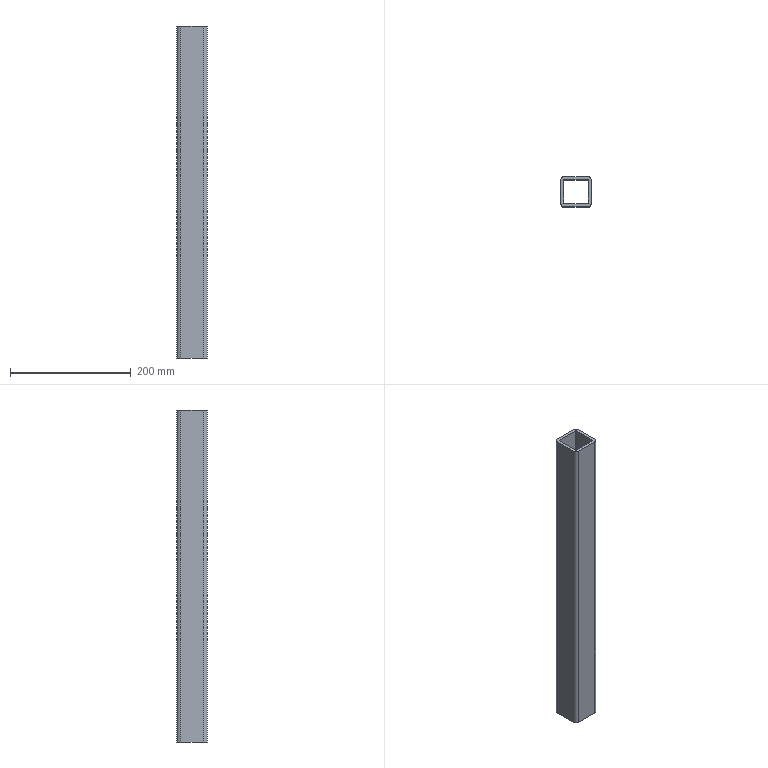Part | SolidWorks | features Extrusion 1 | 1 solid | 18 faces | box 50 x 50 x 550 mm | volume 478476 mm3 | plane 10 | cylinder 8 | commonest cylinder face diameters 2 x4 12 x4
STEP:
#1=CARTESIAN_POINT('',(0.,6.,550.));
#2=VERTEX_POINT('',#1);
#3=CARTESIAN_POINT('',(6.,0.,550.));
#4=VERTEX_POINT('',#3);
#5=CARTESIAN_POINT('',(6.,6.,550.));
#6=DIRECTION('',(0.,0.,1.));
#7=DIRECTION('',(-1.,0.,0.));
#8=AXIS2_PLACEMENT_3D('',#5,#6,#7);
#9=CIRCLE('',#8,6.);
#10=EDGE_CURVE('',#2,#4,#9,.T.);
#11=ORIENTED_EDGE('',*,*,#10,.T.);
#12=CARTESIAN_POINT('',(44.,0.,550.));
#13=VERTEX_POINT('',#12);
#14=CARTESIAN_POINT('',(6.,0.,550.));
#15=DIRECTION('',(1.,0.,0.));
#16=VECTOR('',#15,1000.);
#17=LINE('',#14,#16);
#18=EDGE_CURVE('',#4,#13,#17,.T.);
#19=ORIENTED_EDGE('',*,*,#18,.T.);
#20=CARTESIAN_POINT('',(50.,6.,550.));
#21=VERTEX_POINT('',#20);
#22=CARTESIAN_POINT('',(44.,6.,550.));
#23=DIRECTION('',(0.,0.,1.));
#24=DIRECTION('',(1.,0.,0.));
#25=AXIS2_PLACEMENT_3D('',#22,#23,#24);
#26=CIRCLE('',#25,6.);
#27=EDGE_CURVE('',#13,#21,#26,.T.);
#28=ORIENTED_EDGE('',*,*,#27,.T.);
#29=CARTESIAN_POINT('',(50.,44.,550.));
#30=VERTEX_POINT('',#29);
#31=CARTESIAN_POINT('',(50.,6.,550.));
#32=DIRECTION('',(0.,1.,0.));
#33=VECTOR('',#32,1000.);
#34=LINE('',#31,#33);
#35=EDGE_CURVE('',#21,#30,#34,.T.);
#36=ORIENTED_EDGE('',*,*,#35,.T.);
#37=CARTESIAN_POINT('',(44.,50.,550.));
#38=VERTEX_POINT('',#37);
#39=CARTESIAN_POINT('',(44.,44.,550.));
#40=DIRECTION('',(0.,0.,1.));
#41=DIRECTION('',(-1.,0.,0.));
#42=AXIS2_PLACEMENT_3D('',#39,#40,#41);
#43=CIRCLE('',#42,6.);
#44=EDGE_CURVE('',#30,#38,#43,.T.);
#45=ORIENTED_EDGE('',*,*,#44,.T.);
#46=CARTESIAN_POINT('',(6.,50.,550.));
#47=VERTEX_POINT('',#46);
#48=CARTESIAN_POINT('',(6.,50.,550.));
#49=DIRECTION('',(-1.,0.,0.));
#50=VECTOR('',#49,1000.);
#51=LINE('',#48,#50);
#52=EDGE_CURVE('',#38,#47,#51,.T.);
#53=ORIENTED_EDGE('',*,*,#52,.T.);
#54=CARTESIAN_POINT('',(0.,44.,550.));
#55=VERTEX_POINT('',#54);
#56=CARTESIAN_POINT('',(6.,44.,550.));
#57=DIRECTION('',(0.,0.,1.));
#58=DIRECTION('',(-1.,0.,0.));
#59=AXIS2_PLACEMENT_3D('',#56,#57,#58);
#60=CIRCLE('',#59,6.);
#61=EDGE_CURVE('',#47,#55,#60,.T.);
#62=ORIENTED_EDGE('',*,*,#61,.T.);
#63=CARTESIAN_POINT('',(0.,6.,550.));
#64=DIRECTION('',(0.,-1.,0.));
#65=VECTOR('',#64,1000.);
#66=LINE('',#63,#65);
#67=EDGE_CURVE('',#55,#2,#66,.T.);
#68=ORIENTED_EDGE('',*,*,#67,.T.);
#69=EDGE_LOOP('',(#11,#19,#28,#36,#45,#53,#62,#68));
#70=FACE_OUTER_BOUND('',#69,.T.);
#71=CARTESIAN_POINT('',(6.,45.,550.));
#72=VERTEX_POINT('',#71);
#73=CARTESIAN_POINT('',(5.,44.,550.));
#74=VERTEX_POINT('',#73);
#75=CARTESIAN_POINT('',(6.,44.,550.));
#76=DIRECTION('',(0.,0.,1.));
#77=DIRECTION('',(-1.,0.,0.));
#78=AXIS2_PLACEMENT_3D('',#75,#76,#77);
#79=CIRCLE('',#78,1.);
#80=EDGE_CURVE('',#72,#74,#79,.T.);
#81=ORIENTED_EDGE('',*,*,#80,.F.);
#82=CARTESIAN_POINT('',(44.,45.,550.));
#83=VERTEX_POINT('',#82);
#84=CARTESIAN_POINT('',(6.,45.,550.));
#85=DIRECTION('',(-1.,0.,0.));
#86=VECTOR('',#85,1000.);
#87=LINE('',#84,#86);
#88=EDGE_CURVE('',#83,#72,#87,.T.);
#89=ORIENTED_EDGE('',*,*,#88,.F.);
#90=CARTESIAN_POINT('',(45.,44.,550.));
#91=VERTEX_POINT('',#90);
#92=CARTESIAN_POINT('',(44.,44.,550.));
#93=DIRECTION('',(0.,0.,1.));
#94=DIRECTION('',(-1.,0.,0.));
#95=AXIS2_PLACEMENT_3D('',#92,#93,#94);
#96=CIRCLE('',#95,1.);
#97=EDGE_CURVE('',#91,#83,#96,.T.);
#98=ORIENTED_EDGE('',*,*,#97,.F.);
#99=CARTESIAN_POINT('',(45.,6.,550.));
#100=VERTEX_POINT('',#99);
#101=CARTESIAN_POINT('',(45.,6.,550.));
#102=DIRECTION('',(0.,1.,0.));
#103=VECTOR('',#102,1000.);
#104=LINE('',#101,#103);
#105=EDGE_CURVE('',#100,#91,#104,.T.);
#106=ORIENTED_EDGE('',*,*,#105,.F.);
#107=CARTESIAN_POINT('',(44.,5.,550.));
#108=VERTEX_POINT('',#107);
#109=CARTESIAN_POINT('',(44.,6.,550.));
#110=DIRECTION('',(0.,0.,1.));
#111=DIRECTION('',(1.,0.,0.));
#112=AXIS2_PLACEMENT_3D('',#109,#110,#111);
#113=CIRCLE('',#112,1.);
#114=EDGE_CURVE('',#108,#100,#113,.T.);
#115=ORIENTED_EDGE('',*,*,#114,.F.);
#116=CARTESIAN_POINT('',(6.,5.,550.));
#117=VERTEX_POINT('',#116);
#118=CARTESIAN_POINT('',(6.,5.,550.));
#119=DIRECTION('',(1.,0.,0.));
#120=VECTOR('',#119,1000.);
#121=LINE('',#118,#120);
#122=EDGE_CURVE('',#117,#108,#121,.T.);
#123=ORIENTED_EDGE('',*,*,#122,.F.);
#124=CARTESIAN_POINT('',(5.,6.,550.));
#125=VERTEX_POINT('',#124);
#126=CARTESIAN_POINT('',(6.,6.,550.));
#127=DIRECTION('',(0.,0.,1.));
#128=DIRECTION('',(-1.,0.,0.));
#129=AXIS2_PLACEMENT_3D('',#126,#127,#128);
#130=CIRCLE('',#129,1.);
#131=EDGE_CURVE('',#125,#117,#130,.T.);
#132=ORIENTED_EDGE('',*,*,#131,.F.);
#133=CARTESIAN_POINT('',(5.,6.,550.));
#134=DIRECTION('',(0.,-1.,0.));
#135=VECTOR('',#134,1000.);
#136=LINE('',#133,#135);
#137=EDGE_CURVE('',#74,#125,#136,.T.);
#138=ORIENTED_EDGE('',*,*,#137,.F.);
#139=EDGE_LOOP('',(#81,#89,#98,#106,#115,#123,#132,#138));
#140=FACE_BOUND('',#139,.T.);
#141=CARTESIAN_POINT('',(6.,6.,550.));
#142=DIRECTION('',(0.,0.,-1.));
#143=DIRECTION('',(-1.,0.,0.));
#144=AXIS2_PLACEMENT_3D('',#141,#142,#143);
#145=PLANE('',#144);
#146=ADVANCED_FACE('',(#70,#140),#145,.F.);
#147=CARTESIAN_POINT('',(0.,6.,0.));
#148=VERTEX_POINT('',#147);
#149=CARTESIAN_POINT('',(6.,0.,0.));
#150=VERTEX_POINT('',#149);
#151=CARTESIAN_POINT('',(6.,6.,0.));
#152=DIRECTION('',(0.,0.,1.));
#153=DIRECTION('',(-1.,0.,0.));
#154=AXIS2_PLACEMENT_3D('',#151,#152,#153);
#155=CIRCLE('',#154,6.);
#156=EDGE_CURVE('',#148,#150,#155,.T.);
#157=ORIENTED_EDGE('',*,*,#156,.F.);
#158=CARTESIAN_POINT('',(0.,44.,0.));
#159=VERTEX_POINT('',#158);
#160=CARTESIAN_POINT('',(0.,6.,0.));
#161=DIRECTION('',(0.,-1.,0.));
#162=VECTOR('',#161,1000.);
#163=LINE('',#160,#162);
#164=EDGE_CURVE('',#159,#148,#163,.T.);
#165=ORIENTED_EDGE('',*,*,#164,.F.);
#166=CARTESIAN_POINT('',(6.,50.,0.));
#167=VERTEX_POINT('',#166);
#168=CARTESIAN_POINT('',(6.,44.,0.));
#169=DIRECTION('',(0.,0.,1.));
#170=DIRECTION('',(-1.,0.,0.));
#171=AXIS2_PLACEMENT_3D('',#168,#169,#170);
#172=CIRCLE('',#171,6.);
#173=EDGE_CURVE('',#167,#159,#172,.T.);
#174=ORIENTED_EDGE('',*,*,#173,.F.);
#175=CARTESIAN_POINT('',(44.,50.,0.));
#176=VERTEX_POINT('',#175);
#177=CARTESIAN_POINT('',(6.,50.,0.));
#178=DIRECTION('',(-1.,0.,0.));
#179=VECTOR('',#178,1000.);
#180=LINE('',#177,#179);
#181=EDGE_CURVE('',#176,#167,#180,.T.);
#182=ORIENTED_EDGE('',*,*,#181,.F.);
#183=CARTESIAN_POINT('',(50.,44.,0.));
#184=VERTEX_POINT('',#183);
#185=CARTESIAN_POINT('',(44.,44.,0.));
#186=DIRECTION('',(0.,0.,1.));
#187=DIRECTION('',(-1.,0.,0.));
#188=AXIS2_PLACEMENT_3D('',#185,#186,#187);
#189=CIRCLE('',#188,6.);
#190=EDGE_CURVE('',#184,#176,#189,.T.);
#191=ORIENTED_EDGE('',*,*,#190,.F.);
#192=CARTESIAN_POINT('',(50.,6.,0.));
#193=VERTEX_POINT('',#192);
#194=CARTESIAN_POINT('',(50.,6.,0.));
#195=DIRECTION('',(0.,1.,0.));
#196=VECTOR('',#195,1000.);
#197=LINE('',#194,#196);
#198=EDGE_CURVE('',#193,#184,#197,.T.);
#199=ORIENTED_EDGE('',*,*,#198,.F.);
#200=CARTESIAN_POINT('',(44.,0.,0.));
#201=VERTEX_POINT('',#200);
#202=CARTESIAN_POINT('',(44.,6.,0.));
#203=DIRECTION('',(0.,0.,1.));
#204=DIRECTION('',(1.,0.,0.));
#205=AXIS2_PLACEMENT_3D('',#202,#203,#204);
#206=CIRCLE('',#205,6.);
#207=EDGE_CURVE('',#201,#193,#206,.T.);
#208=ORIENTED_EDGE('',*,*,#207,.F.);
#209=CARTESIAN_POINT('',(6.,0.,0.));
#210=DIRECTION('',(1.,0.,0.));
#211=VECTOR('',#210,1000.);
#212=LINE('',#209,#211);
#213=EDGE_CURVE('',#150,#201,#212,.T.);
#214=ORIENTED_EDGE('',*,*,#213,.F.);
#215=EDGE_LOOP('',(#157,#165,#174,#182,#191,#199,#208,#214));
#216=FACE_OUTER_BOUND('',#215,.T.);
#217=CARTESIAN_POINT('',(44.,45.,0.));
#218=VERTEX_POINT('',#217);
#219=CARTESIAN_POINT('',(6.,45.,0.));
#220=VERTEX_POINT('',#219);
#221=CARTESIAN_POINT('',(6.,45.,0.));
#222=DIRECTION('',(-1.,0.,0.));
#223=VECTOR('',#222,1000.);
#224=LINE('',#221,#223);
#225=EDGE_CURVE('',#218,#220,#224,.T.);
#226=ORIENTED_EDGE('',*,*,#225,.T.);
#227=CARTESIAN_POINT('',(5.,44.,0.));
#228=VERTEX_POINT('',#227);
#229=CARTESIAN_POINT('',(6.,44.,0.));
#230=DIRECTION('',(0.,0.,1.));
#231=DIRECTION('',(-1.,0.,0.));
#232=AXIS2_PLACEMENT_3D('',#229,#230,#231);
#233=CIRCLE('',#232,1.);
#234=EDGE_CURVE('',#220,#228,#233,.T.);
#235=ORIENTED_EDGE('',*,*,#234,.T.);
#236=CARTESIAN_POINT('',(5.,6.,0.));
#237=VERTEX_POINT('',#236);
#238=CARTESIAN_POINT('',(5.,6.,0.));
#239=DIRECTION('',(0.,-1.,0.));
#240=VECTOR('',#239,1000.);
#241=LINE('',#238,#240);
#242=EDGE_CURVE('',#228,#237,#241,.T.);
#243=ORIENTED_EDGE('',*,*,#242,.T.);
#244=CARTESIAN_POINT('',(6.,5.,0.));
#245=VERTEX_POINT('',#244);
#246=CARTESIAN_POINT('',(6.,6.,0.));
#247=DIRECTION('',(0.,0.,1.));
#248=DIRECTION('',(-1.,0.,0.));
#249=AXIS2_PLACEMENT_3D('',#246,#247,#248);
#250=CIRCLE('',#249,1.);
#251=EDGE_CURVE('',#237,#245,#250,.T.);
#252=ORIENTED_EDGE('',*,*,#251,.T.);
#253=CARTESIAN_POINT('',(44.,5.,0.));
#254=VERTEX_POINT('',#253);
#255=CARTESIAN_POINT('',(6.,5.,0.));
#256=DIRECTION('',(1.,0.,0.));
#257=VECTOR('',#256,1000.);
#258=LINE('',#255,#257);
#259=EDGE_CURVE('',#245,#254,#258,.T.);
#260=ORIENTED_EDGE('',*,*,#259,.T.);
#261=CARTESIAN_POINT('',(45.,6.,0.));
#262=VERTEX_POINT('',#261);
#263=CARTESIAN_POINT('',(44.,6.,0.));
#264=DIRECTION('',(0.,0.,1.));
#265=DIRECTION('',(1.,0.,0.));
#266=AXIS2_PLACEMENT_3D('',#263,#264,#265);
#267=CIRCLE('',#266,1.);
#268=EDGE_CURVE('',#254,#262,#267,.T.);
#269=ORIENTED_EDGE('',*,*,#268,.T.);
#270=CARTESIAN_POINT('',(45.,44.,0.));
#271=VERTEX_POINT('',#270);
#272=CARTESIAN_POINT('',(45.,6.,0.));
#273=DIRECTION('',(0.,1.,0.));
#274=VECTOR('',#273,1000.);
#275=LINE('',#272,#274);
#276=EDGE_CURVE('',#262,#271,#275,.T.);
#277=ORIENTED_EDGE('',*,*,#276,.T.);
#278=CARTESIAN_POINT('',(44.,44.,0.));
#279=DIRECTION('',(0.,0.,1.));
#280=DIRECTION('',(-1.,0.,0.));
#281=AXIS2_PLACEMENT_3D('',#278,#279,#280);
#282=CIRCLE('',#281,1.);
#283=EDGE_CURVE('',#271,#218,#282,.T.);
#284=ORIENTED_EDGE('',*,*,#283,.T.);
#285=EDGE_LOOP('',(#226,#235,#243,#252,#260,#269,#277,#284));
#286=FACE_BOUND('',#285,.T.);
#287=CARTESIAN_POINT('',(6.,6.,0.));
#288=DIRECTION('',(0.,0.,-1.));
#289=DIRECTION('',(-1.,0.,0.));
#290=AXIS2_PLACEMENT_3D('',#287,#288,#289);
#291=PLANE('',#290);
#292=ADVANCED_FACE('',(#216,#286),#291,.T.);
#293=ORIENTED_EDGE('',*,*,#156,.T.);
#294=CARTESIAN_POINT('',(6.,0.,550.));
#295=DIRECTION('',(0.,0.,-1.));
#296=VECTOR('',#295,1000.);
#297=LINE('',#294,#296);
#298=EDGE_CURVE('',#4,#150,#297,.T.);
#299=ORIENTED_EDGE('',*,*,#298,.F.);
#300=ORIENTED_EDGE('',*,*,#10,.F.);
#301=CARTESIAN_POINT('',(0.,6.,550.));
#302=DIRECTION('',(0.,0.,-1.));
#303=VECTOR('',#302,1000.);
#304=LINE('',#301,#303);
#305=EDGE_CURVE('',#2,#148,#304,.T.);
#306=ORIENTED_EDGE('',*,*,#305,.T.);
#307=EDGE_LOOP('',(#293,#299,#300,#306));
#308=FACE_OUTER_BOUND('',#307,.T.);
#309=CARTESIAN_POINT('',(6.,6.,550.));
#310=DIRECTION('',(0.,0.,-1.));
#311=DIRECTION('',(-1.,0.,0.));
#312=AXIS2_PLACEMENT_3D('',#309,#310,#311);
#313=CYLINDRICAL_SURFACE('',#312,6.);
#314=ADVANCED_FACE('',(#308),#313,.T.);
#315=ORIENTED_EDGE('',*,*,#213,.T.);
#316=CARTESIAN_POINT('',(44.,0.,550.));
#317=DIRECTION('',(0.,0.,-1.));
#318=VECTOR('',#317,1000.);
#319=LINE('',#316,#318);
#320=EDGE_CURVE('',#13,#201,#319,.T.);
#321=ORIENTED_EDGE('',*,*,#320,.F.);
#322=ORIENTED_EDGE('',*,*,#18,.F.);
#323=ORIENTED_EDGE('',*,*,#298,.T.);
#324=EDGE_LOOP('',(#315,#321,#322,#323));
#325=FACE_OUTER_BOUND('',#324,.T.);
#326=CARTESIAN_POINT('',(6.,0.,550.));
#327=DIRECTION('',(0.,1.,0.));
#328=DIRECTION('',(0.,0.,1.));
#329=AXIS2_PLACEMENT_3D('',#326,#327,#328);
#330=PLANE('',#329);
#331=ADVANCED_FACE('',(#325),#330,.F.);
#332=ORIENTED_EDGE('',*,*,#207,.T.);
#333=CARTESIAN_POINT('',(50.,6.,550.));
#334=DIRECTION('',(0.,0.,-1.));
#335=VECTOR('',#334,1000.);
#336=LINE('',#333,#335);
#337=EDGE_CURVE('',#21,#193,#336,.T.);
#338=ORIENTED_EDGE('',*,*,#337,.F.);
#339=ORIENTED_EDGE('',*,*,#27,.F.);
#340=ORIENTED_EDGE('',*,*,#320,.T.);
#341=EDGE_LOOP('',(#332,#338,#339,#340));
#342=FACE_OUTER_BOUND('',#341,.T.);
#343=CARTESIAN_POINT('',(44.,6.,550.));
#344=DIRECTION('',(0.,0.,-1.));
#345=DIRECTION('',(-1.,0.,0.));
#346=AXIS2_PLACEMENT_3D('',#343,#344,#345);
#347=CYLINDRICAL_SURFACE('',#346,6.);
#348=ADVANCED_FACE('',(#342),#347,.T.);
#349=ORIENTED_EDGE('',*,*,#198,.T.);
#350=CARTESIAN_POINT('',(50.,44.,550.));
#351=DIRECTION('',(0.,0.,-1.));
#352=VECTOR('',#351,1000.);
#353=LINE('',#350,#352);
#354=EDGE_CURVE('',#30,#184,#353,.T.);
#355=ORIENTED_EDGE('',*,*,#354,.F.);
#356=ORIENTED_EDGE('',*,*,#35,.F.);
#357=ORIENTED_EDGE('',*,*,#337,.T.);
#358=EDGE_LOOP('',(#349,#355,#356,#357));
#359=FACE_OUTER_BOUND('',#358,.T.);
#360=CARTESIAN_POINT('',(50.,6.,550.));
#361=DIRECTION('',(-1.,0.,0.));
#362=DIRECTION('',(0.,0.,1.));
#363=AXIS2_PLACEMENT_3D('',#360,#361,#362);
#364=PLANE('',#363);
#365=ADVANCED_FACE('',(#359),#364,.F.);
#366=ORIENTED_EDGE('',*,*,#190,.T.);
#367=CARTESIAN_POINT('',(44.,50.,550.));
#368=DIRECTION('',(0.,0.,-1.));
#369=VECTOR('',#368,1000.);
#370=LINE('',#367,#369);
#371=EDGE_CURVE('',#38,#176,#370,.T.);
#372=ORIENTED_EDGE('',*,*,#371,.F.);
#373=ORIENTED_EDGE('',*,*,#44,.F.);
#374=ORIENTED_EDGE('',*,*,#354,.T.);
#375=EDGE_LOOP('',(#366,#372,#373,#374));
#376=FACE_OUTER_BOUND('',#375,.T.);
#377=CARTESIAN_POINT('',(44.,44.,550.));
#378=DIRECTION('',(0.,0.,-1.));
#379=DIRECTION('',(-1.,0.,0.));
#380=AXIS2_PLACEMENT_3D('',#377,#378,#379);
#381=CYLINDRICAL_SURFACE('',#380,6.);
#382=ADVANCED_FACE('',(#376),#381,.T.);
#383=ORIENTED_EDGE('',*,*,#181,.T.);
#384=CARTESIAN_POINT('',(6.,50.,550.));
#385=DIRECTION('',(0.,0.,-1.));
#386=VECTOR('',#385,1000.);
#387=LINE('',#384,#386);
#388=EDGE_CURVE('',#47,#167,#387,.T.);
#389=ORIENTED_EDGE('',*,*,#388,.F.);
#390=ORIENTED_EDGE('',*,*,#52,.F.);
#391=ORIENTED_EDGE('',*,*,#371,.T.);
#392=EDGE_LOOP('',(#383,#389,#390,#391));
#393=FACE_OUTER_BOUND('',#392,.T.);
#394=CARTESIAN_POINT('',(6.,50.,550.));
#395=DIRECTION('',(0.,-1.,0.));
#396=DIRECTION('',(0.,0.,-1.));
#397=AXIS2_PLACEMENT_3D('',#394,#395,#396);
#398=PLANE('',#397);
#399=ADVANCED_FACE('',(#393),#398,.F.);
#400=ORIENTED_EDGE('',*,*,#173,.T.);
#401=CARTESIAN_POINT('',(0.,44.,550.));
#402=DIRECTION('',(0.,0.,-1.));
#403=VECTOR('',#402,1000.);
#404=LINE('',#401,#403);
#405=EDGE_CURVE('',#55,#159,#404,.T.);
#406=ORIENTED_EDGE('',*,*,#405,.F.);
#407=ORIENTED_EDGE('',*,*,#61,.F.);
#408=ORIENTED_EDGE('',*,*,#388,.T.);
#409=EDGE_LOOP('',(#400,#406,#407,#408));
#410=FACE_OUTER_BOUND('',#409,.T.);
#411=CARTESIAN_POINT('',(6.,44.,550.));
#412=DIRECTION('',(0.,0.,-1.));
#413=DIRECTION('',(-1.,0.,0.));
#414=AXIS2_PLACEMENT_3D('',#411,#412,#413);
#415=CYLINDRICAL_SURFACE('',#414,6.);
#416=ADVANCED_FACE('',(#410),#415,.T.);
#417=ORIENTED_EDGE('',*,*,#164,.T.);
#418=ORIENTED_EDGE('',*,*,#305,.F.);
#419=ORIENTED_EDGE('',*,*,#67,.F.);
#420=ORIENTED_EDGE('',*,*,#405,.T.);
#421=EDGE_LOOP('',(#417,#418,#419,#420));
#422=FACE_OUTER_BOUND('',#421,.T.);
#423=CARTESIAN_POINT('',(0.,6.,550.));
#424=DIRECTION('',(1.,0.,0.));
#425=DIRECTION('',(0.,0.,-1.));
#426=AXIS2_PLACEMENT_3D('',#423,#424,#425);
#427=PLANE('',#426);
#428=ADVANCED_FACE('',(#422),#427,.F.);
#429=ORIENTED_EDGE('',*,*,#234,.F.);
#430=CARTESIAN_POINT('',(6.,45.,550.));
#431=DIRECTION('',(0.,0.,-1.));
#432=VECTOR('',#431,1000.);
#433=LINE('',#430,#432);
#434=EDGE_CURVE('',#72,#220,#433,.T.);
#435=ORIENTED_EDGE('',*,*,#434,.F.);
#436=ORIENTED_EDGE('',*,*,#80,.T.);
#437=CARTESIAN_POINT('',(5.,44.,550.));
#438=DIRECTION('',(0.,0.,-1.));
#439=VECTOR('',#438,1000.);
#440=LINE('',#437,#439);
#441=EDGE_CURVE('',#74,#228,#440,.T.);
#442=ORIENTED_EDGE('',*,*,#441,.T.);
#443=EDGE_LOOP('',(#429,#435,#436,#442));
#444=FACE_OUTER_BOUND('',#443,.T.);
#445=CARTESIAN_POINT('',(6.,44.,550.));
#446=DIRECTION('',(0.,0.,-1.));
#447=DIRECTION('',(-1.,0.,0.));
#448=AXIS2_PLACEMENT_3D('',#445,#446,#447);
#449=CYLINDRICAL_SURFACE('',#448,1.);
#450=ADVANCED_FACE('',(#444),#449,.F.);
#451=ORIENTED_EDGE('',*,*,#242,.F.);
#452=ORIENTED_EDGE('',*,*,#441,.F.);
#453=ORIENTED_EDGE('',*,*,#137,.T.);
#454=CARTESIAN_POINT('',(5.,6.,550.));
#455=DIRECTION('',(0.,0.,-1.));
#456=VECTOR('',#455,1000.);
#457=LINE('',#454,#456);
#458=EDGE_CURVE('',#125,#237,#457,.T.);
#459=ORIENTED_EDGE('',*,*,#458,.T.);
#460=EDGE_LOOP('',(#451,#452,#453,#459));
#461=FACE_OUTER_BOUND('',#460,.T.);
#462=CARTESIAN_POINT('',(5.,6.,550.));
#463=DIRECTION('',(1.,0.,0.));
#464=DIRECTION('',(0.,1.,0.));
#465=AXIS2_PLACEMENT_3D('',#462,#463,#464);
#466=PLANE('',#465);
#467=ADVANCED_FACE('',(#461),#466,.T.);
#468=ORIENTED_EDGE('',*,*,#251,.F.);
#469=ORIENTED_EDGE('',*,*,#458,.F.);
#470=ORIENTED_EDGE('',*,*,#131,.T.);
#471=CARTESIAN_POINT('',(6.,5.,550.));
#472=DIRECTION('',(0.,0.,-1.));
#473=VECTOR('',#472,1000.);
#474=LINE('',#471,#473);
#475=EDGE_CURVE('',#117,#245,#474,.T.);
#476=ORIENTED_EDGE('',*,*,#475,.T.);
#477=EDGE_LOOP('',(#468,#469,#470,#476));
#478=FACE_OUTER_BOUND('',#477,.T.);
#479=CARTESIAN_POINT('',(6.,6.,550.));
#480=DIRECTION('',(0.,0.,-1.));
#481=DIRECTION('',(-1.,0.,0.));
#482=AXIS2_PLACEMENT_3D('',#479,#480,#481);
#483=CYLINDRICAL_SURFACE('',#482,1.);
#484=ADVANCED_FACE('',(#478),#483,.F.);
#485=ORIENTED_EDGE('',*,*,#259,.F.);
#486=ORIENTED_EDGE('',*,*,#475,.F.);
#487=ORIENTED_EDGE('',*,*,#122,.T.);
#488=CARTESIAN_POINT('',(44.,5.,550.));
#489=DIRECTION('',(0.,0.,-1.));
#490=VECTOR('',#489,1000.);
#491=LINE('',#488,#490);
#492=EDGE_CURVE('',#108,#254,#491,.T.);
#493=ORIENTED_EDGE('',*,*,#492,.T.);
#494=EDGE_LOOP('',(#485,#486,#487,#493));
#495=FACE_OUTER_BOUND('',#494,.T.);
#496=CARTESIAN_POINT('',(6.,5.,550.));
#497=DIRECTION('',(0.,1.,0.));
#498=DIRECTION('',(-1.,0.,0.));
#499=AXIS2_PLACEMENT_3D('',#496,#497,#498);
#500=PLANE('',#499);
#501=ADVANCED_FACE('',(#495),#500,.T.);
#502=ORIENTED_EDGE('',*,*,#268,.F.);
#503=ORIENTED_EDGE('',*,*,#492,.F.);
#504=ORIENTED_EDGE('',*,*,#114,.T.);
#505=CARTESIAN_POINT('',(45.,6.,550.));
#506=DIRECTION('',(0.,0.,-1.));
#507=VECTOR('',#506,1000.);
#508=LINE('',#505,#507);
#509=EDGE_CURVE('',#100,#262,#508,.T.);
#510=ORIENTED_EDGE('',*,*,#509,.T.);
#511=EDGE_LOOP('',(#502,#503,#504,#510));
#512=FACE_OUTER_BOUND('',#511,.T.);
#513=CARTESIAN_POINT('',(44.,6.,550.));
#514=DIRECTION('',(0.,0.,-1.));
#515=DIRECTION('',(-1.,0.,0.));
#516=AXIS2_PLACEMENT_3D('',#513,#514,#515);
#517=CYLINDRICAL_SURFACE('',#516,1.);
#518=ADVANCED_FACE('',(#512),#517,.F.);
#519=ORIENTED_EDGE('',*,*,#276,.F.);
#520=ORIENTED_EDGE('',*,*,#509,.F.);
#521=ORIENTED_EDGE('',*,*,#105,.T.);
#522=CARTESIAN_POINT('',(45.,44.,550.));
#523=DIRECTION('',(0.,0.,-1.));
#524=VECTOR('',#523,1000.);
#525=LINE('',#522,#524);
#526=EDGE_CURVE('',#91,#271,#525,.T.);
#527=ORIENTED_EDGE('',*,*,#526,.T.);
#528=EDGE_LOOP('',(#519,#520,#521,#527));
#529=FACE_OUTER_BOUND('',#528,.T.);
#530=CARTESIAN_POINT('',(45.,6.,550.));
#531=DIRECTION('',(-1.,0.,0.));
#532=DIRECTION('',(0.,0.,1.));
#533=AXIS2_PLACEMENT_3D('',#530,#531,#532);
#534=PLANE('',#533);
#535=ADVANCED_FACE('',(#529),#534,.T.);
#536=ORIENTED_EDGE('',*,*,#283,.F.);
#537=ORIENTED_EDGE('',*,*,#526,.F.);
#538=ORIENTED_EDGE('',*,*,#97,.T.);
#539=CARTESIAN_POINT('',(44.,45.,550.));
#540=DIRECTION('',(0.,0.,-1.));
#541=VECTOR('',#540,1000.);
#542=LINE('',#539,#541);
#543=EDGE_CURVE('',#83,#218,#542,.T.);
#544=ORIENTED_EDGE('',*,*,#543,.T.);
#545=EDGE_LOOP('',(#536,#537,#538,#544));
#546=FACE_OUTER_BOUND('',#545,.T.);
#547=CARTESIAN_POINT('',(44.,44.,550.));
#548=DIRECTION('',(0.,0.,-1.));
#549=DIRECTION('',(-1.,0.,0.));
#550=AXIS2_PLACEMENT_3D('',#547,#548,#549);
#551=CYLINDRICAL_SURFACE('',#550,1.);
#552=ADVANCED_FACE('',(#546),#551,.F.);
#553=ORIENTED_EDGE('',*,*,#225,.F.);
#554=ORIENTED_EDGE('',*,*,#543,.F.);
#555=ORIENTED_EDGE('',*,*,#88,.T.);
#556=ORIENTED_EDGE('',*,*,#434,.T.);
#557=EDGE_LOOP('',(#553,#554,#555,#556));
#558=FACE_OUTER_BOUND('',#557,.T.);
#559=CARTESIAN_POINT('',(6.,45.,550.));
#560=DIRECTION('',(0.,-1.,0.));
#561=DIRECTION('',(0.,0.,-1.));
#562=AXIS2_PLACEMENT_3D('',#559,#560,#561);
#563=PLANE('',#562);
#564=ADVANCED_FACE('',(#558),#563,.T.);
#565=CLOSED_SHELL('',(#146,#292,#314,#331,#348,#365,#382,#399,#416,#428,#450,#467,#484,#501,#518,#535,#552,#564));
#566=MANIFOLD_SOLID_BREP('',#565);
#567=CARTESIAN_POINT('',(0.,0.,0.));
#568=DIRECTION('',(0.,0.,1.));
#569=DIRECTION('',(1.,0.,0.));
#570=AXIS2_PLACEMENT_3D('',#567,#568,#569);
#571=(LENGTH_UNIT()NAMED_UNIT(*)SI_UNIT(.MILLI.,.METRE.));
#572=UNCERTAINTY_MEASURE_WITH_UNIT(LENGTH_MEASURE(0.00001),#571,'','');
#573=(NAMED_UNIT(*)PLANE_ANGLE_UNIT()SI_UNIT($,.RADIAN.));
#574=(NAMED_UNIT(*)SI_UNIT($,.STERADIAN.)SOLID_ANGLE_UNIT());
#575=(GEOMETRIC_REPRESENTATION_CONTEXT(3)GLOBAL_UNCERTAINTY_ASSIGNED_CONTEXT((#572))GLOBAL_UNIT_ASSIGNED_CONTEXT((#571,#573,#574))REPRESENTATION_CONTEXT('',''));
#576=ADVANCED_BREP_SHAPE_REPRESENTATION('',(#566,#570),#575);